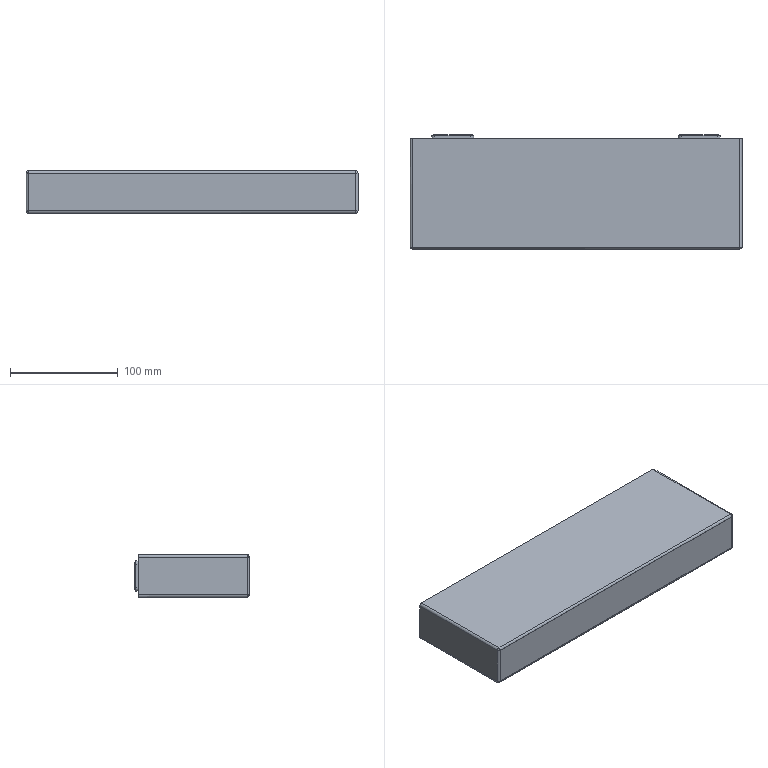Part | STEP file | [CELL]-4 | 1 solid | 75 faces | box 308 x 105.902 x 39.8 mm | volume 1267107 mm3 | cylinder 36 | plane 33 | spline 6 | commonest cylinder face diameters 6 x12 3 x8 4.6 x6 8 x4 10 x4 3.32 x2